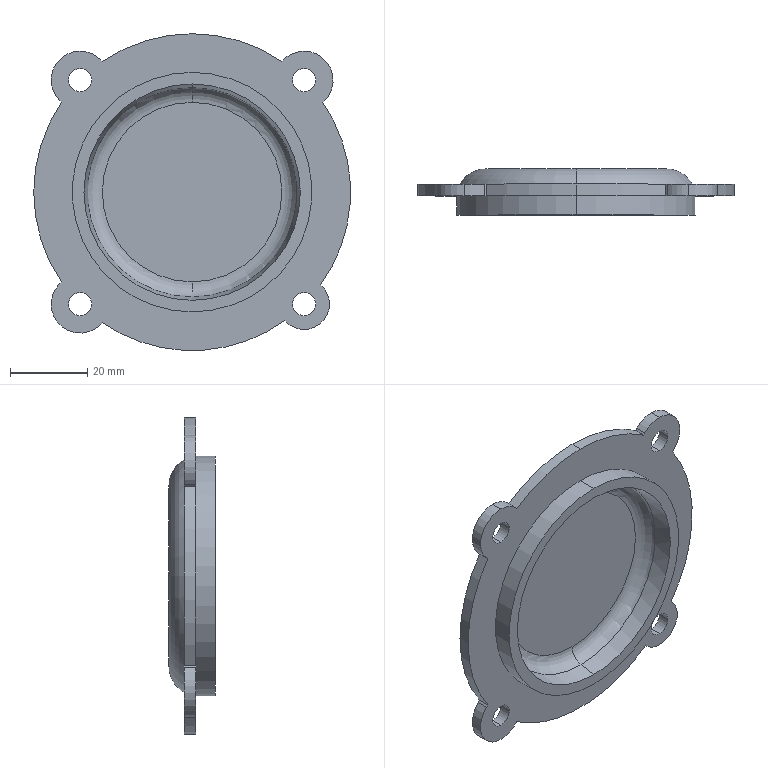Part | SolidWorks | features ICE 2, Revolution 1 | 1 solid | 40 faces | box 82 x 12 x 82 mm | volume 23262 mm3 | cylinder 21 | plane 13 | torus 4 | cone 2 | commonest cylinder face diameters 6 x8 15 x5 82 x5 62 x2 13.12 x1
STEP:
#1=CARTESIAN_POINT('',(-28.991,5.,25.991));
#2=VERTEX_POINT('',#1);
#3=CARTESIAN_POINT('',(-28.991,5.,31.991));
#4=VERTEX_POINT('',#3);
#5=CARTESIAN_POINT('',(-28.991,5.,28.991));
#6=DIRECTION('',(0.,1.,0.));
#7=DIRECTION('',(0.,0.,1.));
#8=AXIS2_PLACEMENT_3D('',#5,#6,#7);
#9=CIRCLE('',#8,3.);
#10=EDGE_CURVE('',#2,#4,#9,.T.);
#11=ORIENTED_EDGE('',*,*,#10,.F.);
#12=CARTESIAN_POINT('',(-28.991,8.,25.991));
#13=VERTEX_POINT('',#12);
#14=CARTESIAN_POINT('',(-28.991,0.,25.991));
#15=DIRECTION('',(0.,1.,0.));
#16=VECTOR('',#15,1000.);
#17=LINE('',#14,#16);
#18=EDGE_CURVE('',#2,#13,#17,.T.);
#19=ORIENTED_EDGE('',*,*,#18,.T.);
#20=CARTESIAN_POINT('',(-28.991,8.,31.991));
#21=VERTEX_POINT('',#20);
#22=CARTESIAN_POINT('',(-28.991,8.,28.991));
#23=DIRECTION('',(0.,1.,0.));
#24=DIRECTION('',(0.,0.,1.));
#25=AXIS2_PLACEMENT_3D('',#22,#23,#24);
#26=CIRCLE('',#25,3.);
#27=EDGE_CURVE('',#13,#21,#26,.T.);
#28=ORIENTED_EDGE('',*,*,#27,.T.);
#29=CARTESIAN_POINT('',(-28.991,0.,31.991));
#30=DIRECTION('',(0.,1.,0.));
#31=VECTOR('',#30,1000.);
#32=LINE('',#29,#31);
#33=EDGE_CURVE('',#4,#21,#32,.T.);
#34=ORIENTED_EDGE('',*,*,#33,.F.);
#35=EDGE_LOOP('',(#11,#19,#28,#34));
#36=FACE_OUTER_BOUND('',#35,.T.);
#37=CARTESIAN_POINT('',(-28.991,0.,28.991));
#38=DIRECTION('',(0.,1.,0.));
#39=DIRECTION('',(0.,0.,1.));
#40=AXIS2_PLACEMENT_3D('',#37,#38,#39);
#41=CYLINDRICAL_SURFACE('',#40,3.);
#42=ADVANCED_FACE('',(#36),#41,.F.);
#43=CARTESIAN_POINT('',(28.991,5.,25.991));
#44=VERTEX_POINT('',#43);
#45=CARTESIAN_POINT('',(28.991,5.,31.991));
#46=VERTEX_POINT('',#45);
#47=CARTESIAN_POINT('',(28.991,5.,28.991));
#48=DIRECTION('',(0.,1.,0.));
#49=DIRECTION('',(0.,0.,1.));
#50=AXIS2_PLACEMENT_3D('',#47,#48,#49);
#51=CIRCLE('',#50,3.);
#52=EDGE_CURVE('',#44,#46,#51,.T.);
#53=ORIENTED_EDGE('',*,*,#52,.F.);
#54=CARTESIAN_POINT('',(28.991,8.,25.991));
#55=VERTEX_POINT('',#54);
#56=CARTESIAN_POINT('',(28.991,0.,25.991));
#57=DIRECTION('',(0.,1.,0.));
#58=VECTOR('',#57,1000.);
#59=LINE('',#56,#58);
#60=EDGE_CURVE('',#44,#55,#59,.T.);
#61=ORIENTED_EDGE('',*,*,#60,.T.);
#62=CARTESIAN_POINT('',(28.991,8.,31.991));
#63=VERTEX_POINT('',#62);
#64=CARTESIAN_POINT('',(28.991,8.,28.991));
#65=DIRECTION('',(0.,1.,0.));
#66=DIRECTION('',(0.,0.,1.));
#67=AXIS2_PLACEMENT_3D('',#64,#65,#66);
#68=CIRCLE('',#67,3.);
#69=EDGE_CURVE('',#55,#63,#68,.T.);
#70=ORIENTED_EDGE('',*,*,#69,.T.);
#71=CARTESIAN_POINT('',(28.991,0.,31.991));
#72=DIRECTION('',(0.,1.,0.));
#73=VECTOR('',#72,1000.);
#74=LINE('',#71,#73);
#75=EDGE_CURVE('',#46,#63,#74,.T.);
#76=ORIENTED_EDGE('',*,*,#75,.F.);
#77=EDGE_LOOP('',(#53,#61,#70,#76));
#78=FACE_OUTER_BOUND('',#77,.T.);
#79=CARTESIAN_POINT('',(28.991,0.,28.991));
#80=DIRECTION('',(0.,1.,0.));
#81=DIRECTION('',(0.,0.,1.));
#82=AXIS2_PLACEMENT_3D('',#79,#80,#81);
#83=CYLINDRICAL_SURFACE('',#82,3.);
#84=ADVANCED_FACE('',(#78),#83,.F.);
#85=CARTESIAN_POINT('',(28.991,5.,-31.991));
#86=VERTEX_POINT('',#85);
#87=CARTESIAN_POINT('',(28.991,5.,-25.991));
#88=VERTEX_POINT('',#87);
#89=CARTESIAN_POINT('',(28.991,5.,-28.991));
#90=DIRECTION('',(0.,1.,0.));
#91=DIRECTION('',(0.,0.,1.));
#92=AXIS2_PLACEMENT_3D('',#89,#90,#91);
#93=CIRCLE('',#92,3.);
#94=EDGE_CURVE('',#86,#88,#93,.T.);
#95=ORIENTED_EDGE('',*,*,#94,.F.);
#96=CARTESIAN_POINT('',(28.991,8.,-31.991));
#97=VERTEX_POINT('',#96);
#98=CARTESIAN_POINT('',(28.991,0.,-31.991));
#99=DIRECTION('',(0.,1.,0.));
#100=VECTOR('',#99,1000.);
#101=LINE('',#98,#100);
#102=EDGE_CURVE('',#86,#97,#101,.T.);
#103=ORIENTED_EDGE('',*,*,#102,.T.);
#104=CARTESIAN_POINT('',(28.991,8.,-25.991));
#105=VERTEX_POINT('',#104);
#106=CARTESIAN_POINT('',(28.991,8.,-28.991));
#107=DIRECTION('',(0.,1.,0.));
#108=DIRECTION('',(0.,0.,1.));
#109=AXIS2_PLACEMENT_3D('',#106,#107,#108);
#110=CIRCLE('',#109,3.);
#111=EDGE_CURVE('',#97,#105,#110,.T.);
#112=ORIENTED_EDGE('',*,*,#111,.T.);
#113=CARTESIAN_POINT('',(28.991,0.,-25.991));
#114=DIRECTION('',(0.,1.,0.));
#115=VECTOR('',#114,1000.);
#116=LINE('',#113,#115);
#117=EDGE_CURVE('',#88,#105,#116,.T.);
#118=ORIENTED_EDGE('',*,*,#117,.F.);
#119=EDGE_LOOP('',(#95,#103,#112,#118));
#120=FACE_OUTER_BOUND('',#119,.T.);
#121=CARTESIAN_POINT('',(28.991,0.,-28.991));
#122=DIRECTION('',(0.,1.,0.));
#123=DIRECTION('',(0.,0.,1.));
#124=AXIS2_PLACEMENT_3D('',#121,#122,#123);
#125=CYLINDRICAL_SURFACE('',#124,3.);
#126=ADVANCED_FACE('',(#120),#125,.F.);
#127=CARTESIAN_POINT('',(-28.991,5.,-31.991));
#128=VERTEX_POINT('',#127);
#129=CARTESIAN_POINT('',(-28.991,5.,-25.991));
#130=VERTEX_POINT('',#129);
#131=CARTESIAN_POINT('',(-28.991,5.,-28.991));
#132=DIRECTION('',(0.,1.,0.));
#133=DIRECTION('',(0.,0.,1.));
#134=AXIS2_PLACEMENT_3D('',#131,#132,#133);
#135=CIRCLE('',#134,3.);
#136=EDGE_CURVE('',#128,#130,#135,.T.);
#137=ORIENTED_EDGE('',*,*,#136,.F.);
#138=CARTESIAN_POINT('',(-28.991,8.,-31.991));
#139=VERTEX_POINT('',#138);
#140=CARTESIAN_POINT('',(-28.991,0.,-31.991));
#141=DIRECTION('',(0.,1.,0.));
#142=VECTOR('',#141,1000.);
#143=LINE('',#140,#142);
#144=EDGE_CURVE('',#128,#139,#143,.T.);
#145=ORIENTED_EDGE('',*,*,#144,.T.);
#146=CARTESIAN_POINT('',(-28.991,8.,-25.991));
#147=VERTEX_POINT('',#146);
#148=CARTESIAN_POINT('',(-28.991,8.,-28.991));
#149=DIRECTION('',(0.,1.,0.));
#150=DIRECTION('',(0.,0.,1.));
#151=AXIS2_PLACEMENT_3D('',#148,#149,#150);
#152=CIRCLE('',#151,3.);
#153=EDGE_CURVE('',#139,#147,#152,.T.);
#154=ORIENTED_EDGE('',*,*,#153,.T.);
#155=CARTESIAN_POINT('',(-28.991,0.,-25.991));
#156=DIRECTION('',(0.,1.,0.));
#157=VECTOR('',#156,1000.);
#158=LINE('',#155,#157);
#159=EDGE_CURVE('',#130,#147,#158,.T.);
#160=ORIENTED_EDGE('',*,*,#159,.F.);
#161=EDGE_LOOP('',(#137,#145,#154,#160));
#162=FACE_OUTER_BOUND('',#161,.T.);
#163=CARTESIAN_POINT('',(-28.991,0.,-28.991));
#164=DIRECTION('',(0.,1.,0.));
#165=DIRECTION('',(0.,0.,1.));
#166=AXIS2_PLACEMENT_3D('',#163,#164,#165);
#167=CYLINDRICAL_SURFACE('',#166,3.);
#168=ADVANCED_FACE('',(#162),#167,.F.);
#169=CARTESIAN_POINT('',(23.681,5.,34.287));
#170=VERTEX_POINT('',#169);
#171=CARTESIAN_POINT('',(28.991,5.,36.491));
#172=VERTEX_POINT('',#171);
#173=CARTESIAN_POINT('',(28.991,5.,28.991));
#174=DIRECTION('',(0.,1.,0.));
#175=DIRECTION('',(0.,0.,1.));
#176=AXIS2_PLACEMENT_3D('',#173,#174,#175);
#177=CIRCLE('',#176,7.5);
#178=EDGE_CURVE('',#170,#172,#177,.T.);
#179=ORIENTED_EDGE('',*,*,#178,.T.);
#180=CARTESIAN_POINT('',(28.991,8.,36.491));
#181=VERTEX_POINT('',#180);
#182=CARTESIAN_POINT('',(28.991,5.,36.491));
#183=DIRECTION('',(0.,1.,0.));
#184=VECTOR('',#183,1000.);
#185=LINE('',#182,#184);
#186=EDGE_CURVE('',#172,#181,#185,.T.);
#187=ORIENTED_EDGE('',*,*,#186,.T.);
#188=CARTESIAN_POINT('',(23.681,8.,34.287));
#189=VERTEX_POINT('',#188);
#190=CARTESIAN_POINT('',(28.991,8.,28.991));
#191=DIRECTION('',(0.,1.,0.));
#192=DIRECTION('',(0.,0.,1.));
#193=AXIS2_PLACEMENT_3D('',#190,#191,#192);
#194=CIRCLE('',#193,7.5);
#195=EDGE_CURVE('',#189,#181,#194,.T.);
#196=ORIENTED_EDGE('',*,*,#195,.F.);
#197=CARTESIAN_POINT('',(23.681,5.,34.287));
#198=DIRECTION('',(0.,1.,0.));
#199=VECTOR('',#198,1000.);
#200=LINE('',#197,#199);
#201=EDGE_CURVE('',#170,#189,#200,.T.);
#202=ORIENTED_EDGE('',*,*,#201,.F.);
#203=EDGE_LOOP('',(#179,#187,#196,#202));
#204=FACE_OUTER_BOUND('',#203,.T.);
#205=CARTESIAN_POINT('',(28.991,5.,28.991));
#206=DIRECTION('',(0.,1.,0.));
#207=DIRECTION('',(0.,0.,1.));
#208=AXIS2_PLACEMENT_3D('',#205,#206,#207);
#209=CYLINDRICAL_SURFACE('',#208,7.5);
#210=ADVANCED_FACE('',(#204),#209,.T.);
#211=CARTESIAN_POINT('',(-34.234,5.,23.628));
#212=VERTEX_POINT('',#211);
#213=CARTESIAN_POINT('',(-28.991,5.,36.491));
#214=VERTEX_POINT('',#213);
#215=CARTESIAN_POINT('',(-28.991,5.,28.991));
#216=DIRECTION('',(0.,1.,0.));
#217=DIRECTION('',(0.,0.,1.));
#218=AXIS2_PLACEMENT_3D('',#215,#216,#217);
#219=CIRCLE('',#218,7.5);
#220=EDGE_CURVE('',#212,#214,#219,.T.);
#221=ORIENTED_EDGE('',*,*,#220,.T.);
#222=CARTESIAN_POINT('',(-28.991,8.,36.491));
#223=VERTEX_POINT('',#222);
#224=CARTESIAN_POINT('',(-28.991,5.,36.491));
#225=DIRECTION('',(0.,1.,0.));
#226=VECTOR('',#225,1000.);
#227=LINE('',#224,#226);
#228=EDGE_CURVE('',#214,#223,#227,.T.);
#229=ORIENTED_EDGE('',*,*,#228,.T.);
#230=CARTESIAN_POINT('',(-34.234,8.,23.628));
#231=VERTEX_POINT('',#230);
#232=CARTESIAN_POINT('',(-28.991,8.,28.991));
#233=DIRECTION('',(0.,1.,0.));
#234=DIRECTION('',(0.,0.,1.));
#235=AXIS2_PLACEMENT_3D('',#232,#233,#234);
#236=CIRCLE('',#235,7.5);
#237=EDGE_CURVE('',#231,#223,#236,.T.);
#238=ORIENTED_EDGE('',*,*,#237,.F.);
#239=CARTESIAN_POINT('',(-34.234,5.,23.628));
#240=DIRECTION('',(0.,1.,0.));
#241=VECTOR('',#240,1000.);
#242=LINE('',#239,#241);
#243=EDGE_CURVE('',#212,#231,#242,.T.);
#244=ORIENTED_EDGE('',*,*,#243,.F.);
#245=EDGE_LOOP('',(#221,#229,#238,#244));
#246=FACE_OUTER_BOUND('',#245,.T.);
#247=CARTESIAN_POINT('',(-28.991,5.,28.991));
#248=DIRECTION('',(0.,1.,0.));
#249=DIRECTION('',(0.,0.,1.));
#250=AXIS2_PLACEMENT_3D('',#247,#248,#249);
#251=CYLINDRICAL_SURFACE('',#250,7.5);
#252=ADVANCED_FACE('',(#246),#251,.T.);
#253=CARTESIAN_POINT('',(0.,4.695,-27.172));
#254=VERTEX_POINT('',#253);
#255=CARTESIAN_POINT('',(0.,4.695,27.172));
#256=VERTEX_POINT('',#255);
#257=CARTESIAN_POINT('',(0.,4.695,0.));
#258=DIRECTION('',(0.,1.,0.));
#259=DIRECTION('',(0.,0.,1.));
#260=AXIS2_PLACEMENT_3D('',#257,#258,#259);
#261=CIRCLE('',#260,27.172);
#262=EDGE_CURVE('',#254,#256,#261,.T.);
#263=ORIENTED_EDGE('',*,*,#262,.F.);
#264=CARTESIAN_POINT('',(0.,8.,-23.233));
#265=VERTEX_POINT('',#264);
#266=CARTESIAN_POINT('',(0.,4.,-23.233));
#267=DIRECTION('',(1.,0.,0.));
#268=DIRECTION('',(0.,0.,-1.));
#269=AXIS2_PLACEMENT_3D('',#266,#267,#268);
#270=CIRCLE('',#269,4.);
#271=EDGE_CURVE('',#254,#265,#270,.T.);
#272=ORIENTED_EDGE('',*,*,#271,.T.);
#273=CARTESIAN_POINT('',(0.,8.,23.233));
#274=VERTEX_POINT('',#273);
#275=CARTESIAN_POINT('',(0.,8.,0.));
#276=DIRECTION('',(0.,1.,0.));
#277=DIRECTION('',(0.,0.,1.));
#278=AXIS2_PLACEMENT_3D('',#275,#276,#277);
#279=CIRCLE('',#278,23.233);
#280=EDGE_CURVE('',#265,#274,#279,.T.);
#281=ORIENTED_EDGE('',*,*,#280,.T.);
#282=CARTESIAN_POINT('',(0.,4.,23.233));
#283=DIRECTION('',(-1.,0.,0.));
#284=DIRECTION('',(0.,0.,1.));
#285=AXIS2_PLACEMENT_3D('',#282,#283,#284);
#286=CIRCLE('',#285,4.);
#287=EDGE_CURVE('',#256,#274,#286,.T.);
#288=ORIENTED_EDGE('',*,*,#287,.F.);
#289=EDGE_LOOP('',(#263,#272,#281,#288));
#290=FACE_OUTER_BOUND('',#289,.T.);
#291=CARTESIAN_POINT('',(0.,4.,0.));
#292=DIRECTION('',(0.,1.,0.));
#293=DIRECTION('',(0.,0.,1.));
#294=AXIS2_PLACEMENT_3D('',#291,#292,#293);
#295=TOROIDAL_SURFACE('',#294,23.233,4.);
#296=ADVANCED_FACE('',(#290),#295,.F.);
#297=CARTESIAN_POINT('',(0.,8.,30.161));
#298=VERTEX_POINT('',#297);
#299=CARTESIAN_POINT('',(0.,8.,-30.161));
#300=VERTEX_POINT('',#299);
#301=CARTESIAN_POINT('',(0.,8.,0.));
#302=DIRECTION('',(0.,1.,0.));
#303=DIRECTION('',(0.,0.,1.));
#304=AXIS2_PLACEMENT_3D('',#301,#302,#303);
#305=CIRCLE('',#304,30.161);
#306=EDGE_CURVE('',#298,#300,#305,.T.);
#307=ORIENTED_EDGE('',*,*,#306,.T.);
#308=CARTESIAN_POINT('',(0.,12.,-23.233));
#309=VERTEX_POINT('',#308);
#310=CARTESIAN_POINT('',(0.,4.,-23.233));
#311=DIRECTION('',(1.,0.,0.));
#312=DIRECTION('',(0.,0.,-1.));
#313=AXIS2_PLACEMENT_3D('',#310,#311,#312);
#314=CIRCLE('',#313,8.);
#315=EDGE_CURVE('',#300,#309,#314,.T.);
#316=ORIENTED_EDGE('',*,*,#315,.T.);
#317=CARTESIAN_POINT('',(0.,12.,23.233));
#318=VERTEX_POINT('',#317);
#319=CARTESIAN_POINT('',(0.,12.,0.));
#320=DIRECTION('',(0.,1.,0.));
#321=DIRECTION('',(0.,0.,1.));
#322=AXIS2_PLACEMENT_3D('',#319,#320,#321);
#323=CIRCLE('',#322,23.233);
#324=EDGE_CURVE('',#318,#309,#323,.T.);
#325=ORIENTED_EDGE('',*,*,#324,.F.);
#326=CARTESIAN_POINT('',(0.,4.,23.233));
#327=DIRECTION('',(-1.,0.,0.));
#328=DIRECTION('',(0.,0.,1.));
#329=AXIS2_PLACEMENT_3D('',#326,#327,#328);
#330=CIRCLE('',#329,8.);
#331=EDGE_CURVE('',#298,#318,#330,.T.);
#332=ORIENTED_EDGE('',*,*,#331,.F.);
#333=EDGE_LOOP('',(#307,#316,#325,#332));
#334=FACE_OUTER_BOUND('',#333,.T.);
#335=CARTESIAN_POINT('',(0.,4.,0.));
#336=DIRECTION('',(0.,1.,0.));
#337=DIRECTION('',(0.,0.,1.));
#338=AXIS2_PLACEMENT_3D('',#335,#336,#337);
#339=TOROIDAL_SURFACE('',#338,23.233,8.);
#340=ADVANCED_FACE('',(#334),#339,.T.);
#341=CARTESIAN_POINT('',(0.,0.,31.));
#342=VERTEX_POINT('',#341);
#343=CARTESIAN_POINT('',(0.,0.,-31.));
#344=VERTEX_POINT('',#343);
#345=CARTESIAN_POINT('',(0.,0.,0.));
#346=DIRECTION('',(0.,1.,0.));
#347=DIRECTION('',(0.,0.,1.));
#348=AXIS2_PLACEMENT_3D('',#345,#346,#347);
#349=CIRCLE('',#348,31.);
#350=EDGE_CURVE('',#342,#344,#349,.T.);
#351=ORIENTED_EDGE('',*,*,#350,.T.);
#352=CARTESIAN_POINT('',(0.,5.,-31.));
#353=VERTEX_POINT('',#352);
#354=CARTESIAN_POINT('',(0.,53.941,-31.));
#355=DIRECTION('',(0.,1.,0.));
#356=VECTOR('',#355,1000.);
#357=LINE('',#354,#356);
#358=EDGE_CURVE('',#344,#353,#357,.T.);
#359=ORIENTED_EDGE('',*,*,#358,.T.);
#360=CARTESIAN_POINT('',(0.,5.,31.));
#361=VERTEX_POINT('',#360);
#362=CARTESIAN_POINT('',(0.,5.,0.));
#363=DIRECTION('',(0.,1.,0.));
#364=DIRECTION('',(0.,0.,1.));
#365=AXIS2_PLACEMENT_3D('',#362,#363,#364);
#366=CIRCLE('',#365,31.);
#367=EDGE_CURVE('',#361,#353,#366,.T.);
#368=ORIENTED_EDGE('',*,*,#367,.F.);
#369=CARTESIAN_POINT('',(0.,53.941,31.));
#370=DIRECTION('',(0.,1.,0.));
#371=VECTOR('',#370,1000.);
#372=LINE('',#369,#371);
#373=EDGE_CURVE('',#342,#361,#372,.T.);
#374=ORIENTED_EDGE('',*,*,#373,.F.);
#375=EDGE_LOOP('',(#351,#359,#368,#374));
#376=FACE_OUTER_BOUND('',#375,.T.);
#377=CARTESIAN_POINT('',(0.,53.941,0.));
#378=DIRECTION('',(0.,1.,0.));
#379=DIRECTION('',(0.,0.,1.));
#380=AXIS2_PLACEMENT_3D('',#377,#378,#379);
#381=CYLINDRICAL_SURFACE('',#380,31.);
#382=ADVANCED_FACE('',(#376),#381,.T.);
#383=ORIENTED_EDGE('',*,*,#262,.T.);
#384=CARTESIAN_POINT('',(0.,0.,28.));
#385=VERTEX_POINT('',#384);
#386=CARTESIAN_POINT('',(0.,4.695,27.172));
#387=DIRECTION('',(0.,-0.9848,0.1736));
#388=VECTOR('',#387,1000.);
#389=LINE('',#386,#388);
#390=EDGE_CURVE('',#256,#385,#389,.T.);
#391=ORIENTED_EDGE('',*,*,#390,.T.);
#392=CARTESIAN_POINT('',(0.,0.,-28.));
#393=VERTEX_POINT('',#392);
#394=CARTESIAN_POINT('',(0.,0.,0.));
#395=DIRECTION('',(0.,1.,0.));
#396=DIRECTION('',(0.,0.,1.));
#397=AXIS2_PLACEMENT_3D('',#394,#395,#396);
#398=CIRCLE('',#397,28.);
#399=EDGE_CURVE('',#393,#385,#398,.T.);
#400=ORIENTED_EDGE('',*,*,#399,.F.);
#401=CARTESIAN_POINT('',(0.,4.695,-27.172));
#402=DIRECTION('',(0.,-0.9848,-0.1736));
#403=VECTOR('',#402,1000.);
#404=LINE('',#401,#403);
#405=EDGE_CURVE('',#254,#393,#404,.T.);
#406=ORIENTED_EDGE('',*,*,#405,.F.);
#407=EDGE_LOOP('',(#383,#391,#400,#406));
#408=FACE_OUTER_BOUND('',#407,.T.);
#409=CARTESIAN_POINT('',(0.,4.695,0.));
#410=DIRECTION('',(0.,-1.,0.));
#411=DIRECTION('',(0.,0.,-1.));
#412=AXIS2_PLACEMENT_3D('',#409,#410,#411);
#413=CONICAL_SURFACE('',#412,27.172,0.1745);
#414=ADVANCED_FACE('',(#408),#413,.F.);
#415=CARTESIAN_POINT('',(-23.205,5.,33.801));
#416=VERTEX_POINT('',#415);
#417=CARTESIAN_POINT('',(0.,5.,41.));
#418=VERTEX_POINT('',#417);
#419=CARTESIAN_POINT('',(0.,5.,0.));
#420=DIRECTION('',(0.,1.,0.));
#421=DIRECTION('',(0.,0.,1.));
#422=AXIS2_PLACEMENT_3D('',#419,#420,#421);
#423=CIRCLE('',#422,41.);
#424=EDGE_CURVE('',#416,#418,#423,.T.);
#425=ORIENTED_EDGE('',*,*,#424,.T.);
#426=CARTESIAN_POINT('',(0.,8.,41.));
#427=VERTEX_POINT('',#426);
#428=CARTESIAN_POINT('',(0.,53.941,41.));
#429=DIRECTION('',(0.,1.,0.));
#430=VECTOR('',#429,1000.);
#431=LINE('',#428,#430);
#432=EDGE_CURVE('',#418,#427,#431,.T.);
#433=ORIENTED_EDGE('',*,*,#432,.T.);
#434=CARTESIAN_POINT('',(-23.205,8.,33.801));
#435=VERTEX_POINT('',#434);
#436=CARTESIAN_POINT('',(0.,8.,0.));
#437=DIRECTION('',(0.,1.,0.));
#438=DIRECTION('',(0.,0.,1.));
#439=AXIS2_PLACEMENT_3D('',#436,#437,#438);
#440=CIRCLE('',#439,41.);
#441=EDGE_CURVE('',#435,#427,#440,.T.);
#442=ORIENTED_EDGE('',*,*,#441,.F.);
#443=CARTESIAN_POINT('',(-23.205,5.,33.801));
#444=DIRECTION('',(0.,1.,0.));
#445=VECTOR('',#444,1000.);
#446=LINE('',#443,#445);
#447=EDGE_CURVE('',#416,#435,#446,.T.);
#448=ORIENTED_EDGE('',*,*,#447,.F.);
#449=EDGE_LOOP('',(#425,#433,#442,#448));
#450=FACE_OUTER_BOUND('',#449,.T.);
#451=CARTESIAN_POINT('',(0.,53.941,0.));
#452=DIRECTION('',(0.,1.,0.));
#453=DIRECTION('',(0.,0.,1.));
#454=AXIS2_PLACEMENT_3D('',#451,#452,#453);
#455=CYLINDRICAL_SURFACE('',#454,41.);
#456=ADVANCED_FACE('',(#450),#455,.T.);
#457=ORIENTED_EDGE('',*,*,#432,.F.);
#458=CARTESIAN_POINT('',(23.199,5.,33.805));
#459=VERTEX_POINT('',#458);
#460=CARTESIAN_POINT('',(0.,5.,0.));
#461=DIRECTION('',(0.,1.,0.));
#462=DIRECTION('',(0.,0.,1.));
#463=AXIS2_PLACEMENT_3D('',#460,#461,#462);
#464=CIRCLE('',#463,41.);
#465=EDGE_CURVE('',#418,#459,#464,.T.);
#466=ORIENTED_EDGE('',*,*,#465,.T.);
#467=CARTESIAN_POINT('',(23.199,8.,33.805));
#468=VERTEX_POINT('',#467);
#469=CARTESIAN_POINT('',(23.199,5.,33.805));
#470=DIRECTION('',(0.,1.,0.));
#471=VECTOR('',#470,1000.);
#472=LINE('',#469,#471);
#473=EDGE_CURVE('',#459,#468,#472,.T.);
#474=ORIENTED_EDGE('',*,*,#473,.T.);
#475=CARTESIAN_POINT('',(0.,8.,0.));
#476=DIRECTION('',(0.,1.,0.));
#477=DIRECTION('',(0.,0.,1.));
#478=AXIS2_PLACEMENT_3D('',#475,#476,#477);
#479=CIRCLE('',#478,41.);
#480=EDGE_CURVE('',#427,#468,#479,.T.);
#481=ORIENTED_EDGE('',*,*,#480,.F.);
#482=EDGE_LOOP('',(#457,#466,#474,#481));
#483=FACE_OUTER_BOUND('',#482,.T.);
#484=CARTESIAN_POINT('',(0.,53.941,0.));
#485=DIRECTION('',(0.,1.,0.));
#486=DIRECTION('',(0.,0.,1.));
#487=AXIS2_PLACEMENT_3D('',#484,#485,#486);
#488=CYLINDRICAL_SURFACE('',#487,41.);
#489=ADVANCED_FACE('',(#483),#488,.T.);
#490=CARTESIAN_POINT('',(-33.805,5.,-23.199));
#491=VERTEX_POINT('',#490);
#492=CARTESIAN_POINT('',(-33.801,5.,23.205));
#493=VERTEX_POINT('',#492);
#494=CARTESIAN_POINT('',(0.,5.,0.));
#495=DIRECTION('',(0.,1.,0.));
#496=DIRECTION('',(0.,0.,1.));
#497=AXIS2_PLACEMENT_3D('',#494,#495,#496);
#498=CIRCLE('',#497,41.);
#499=EDGE_CURVE('',#491,#493,#498,.T.);
#500=ORIENTED_EDGE('',*,*,#499,.T.);
#501=CARTESIAN_POINT('',(-33.801,8.,23.205));
#502=VERTEX_POINT('',#501);
#503=CARTESIAN_POINT('',(-33.801,5.,23.205));
#504=DIRECTION('',(0.,1.,0.));
#505=VECTOR('',#504,1000.);
#506=LINE('',#503,#505);
#507=EDGE_CURVE('',#493,#502,#506,.T.);
#508=ORIENTED_EDGE('',*,*,#507,.T.);
#509=CARTESIAN_POINT('',(-33.805,8.,-23.199));
#510=VERTEX_POINT('',#509);
#511=CARTESIAN_POINT('',(0.,8.,0.));
#512=DIRECTION('',(0.,1.,0.));
#513=DIRECTION('',(0.,0.,1.));
#514=AXIS2_PLACEMENT_3D('',#511,#512,#513);
#515=CIRCLE('',#514,41.);
#516=EDGE_CURVE('',#510,#502,#515,.T.);
#517=ORIENTED_EDGE('',*,*,#516,.F.);
#518=CARTESIAN_POINT('',(-33.805,5.,-23.199));
#519=DIRECTION('',(0.,1.,0.));
#520=VECTOR('',#519,1000.);
#521=LINE('',#518,#520);
#522=EDGE_CURVE('',#491,#510,#521,.T.);
#523=ORIENTED_EDGE('',*,*,#522,.F.);
#524=EDGE_LOOP('',(#500,#508,#517,#523));
#525=FACE_OUTER_BOUND('',#524,.T.);
#526=CARTESIAN_POINT('',(0.,53.941,0.));
#527=DIRECTION('',(0.,1.,0.));
#528=DIRECTION('',(0.,0.,1.));
#529=AXIS2_PLACEMENT_3D('',#526,#527,#528);
#530=CYLINDRICAL_SURFACE('',#529,41.);
#531=ADVANCED_FACE('',(#525),#530,.T.);
#532=CARTESIAN_POINT('',(23.974,5.,-33.26));
#533=VERTEX_POINT('',#532);
#534=CARTESIAN_POINT('',(-23.204,5.,-33.802));
#535=VERTEX_POINT('',#534);
#536=CARTESIAN_POINT('',(0.,5.,0.));
#537=DIRECTION('',(0.,1.,0.));
#538=DIRECTION('',(0.,0.,1.));
#539=AXIS2_PLACEMENT_3D('',#536,#537,#538);
#540=CIRCLE('',#539,41.);
#541=EDGE_CURVE('',#533,#535,#540,.T.);
#542=ORIENTED_EDGE('',*,*,#541,.T.);
#543=CARTESIAN_POINT('',(-23.204,8.,-33.802));
#544=VERTEX_POINT('',#543);
#545=CARTESIAN_POINT('',(-23.204,5.,-33.802));
#546=DIRECTION('',(0.,1.,0.));
#547=VECTOR('',#546,1000.);
#548=LINE('',#545,#547);
#549=EDGE_CURVE('',#535,#544,#548,.T.);
#550=ORIENTED_EDGE('',*,*,#549,.T.);
#551=CARTESIAN_POINT('',(23.974,8.,-33.26));
#552=VERTEX_POINT('',#551);
#553=CARTESIAN_POINT('',(0.,8.,0.));
#554=DIRECTION('',(0.,1.,0.));
#555=DIRECTION('',(0.,0.,1.));
#556=AXIS2_PLACEMENT_3D('',#553,#554,#555);
#557=CIRCLE('',#556,41.);
#558=EDGE_CURVE('',#552,#544,#557,.T.);
#559=ORIENTED_EDGE('',*,*,#558,.F.);
#560=CARTESIAN_POINT('',(23.974,5.,-33.26));
#561=DIRECTION('',(0.,1.,0.));
#562=VECTOR('',#561,1000.);
#563=LINE('',#560,#562);
#564=EDGE_CURVE('',#533,#552,#563,.T.);
#565=ORIENTED_EDGE('',*,*,#564,.F.);
#566=EDGE_LOOP('',(#542,#550,#559,#565));
#567=FACE_OUTER_BOUND('',#566,.T.);
#568=CARTESIAN_POINT('',(0.,53.941,0.));
#569=DIRECTION('',(0.,1.,0.));
#570=DIRECTION('',(0.,0.,1.));
#571=AXIS2_PLACEMENT_3D('',#568,#569,#570);
#572=CYLINDRICAL_SURFACE('',#571,41.);
#573=ADVANCED_FACE('',(#567),#572,.T.);
#574=ORIENTED_EDGE('',*,*,#390,.F.);
#575=CARTESIAN_POINT('',(0.,4.695,0.));
#576=DIRECTION('',(0.,1.,0.));
#577=DIRECTION('',(0.,0.,1.));
#578=AXIS2_PLACEMENT_3D('',#575,#576,#577);
#579=CIRCLE('',#578,27.172);
#580=EDGE_CURVE('',#256,#254,#579,.T.);
#581=ORIENTED_EDGE('',*,*,#580,.T.);
#582=ORIENTED_EDGE('',*,*,#405,.T.);
#583=CARTESIAN_POINT('',(0.,0.,0.));
#584=DIRECTION('',(0.,1.,0.));
#585=DIRECTION('',(0.,0.,1.));
#586=AXIS2_PLACEMENT_3D('',#583,#584,#585);
#587=CIRCLE('',#586,28.);
#588=EDGE_CURVE('',#385,#393,#587,.T.);
#589=ORIENTED_EDGE('',*,*,#588,.F.);
#590=EDGE_LOOP('',(#574,#581,#582,#589));
#591=FACE_OUTER_BOUND('',#590,.T.);
#592=CARTESIAN_POINT('',(0.,4.695,0.));
#593=DIRECTION('',(0.,-1.,0.));
#594=DIRECTION('',(0.,0.,-1.));
#595=AXIS2_PLACEMENT_3D('',#592,#593,#594);
#596=CONICAL_SURFACE('',#595,27.172,0.1745);
#597=ADVANCED_FACE('',(#591),#596,.F.);
#598=ORIENTED_EDGE('',*,*,#350,.F.);
#599=CARTESIAN_POINT('',(0.,0.,0.));
#600=DIRECTION('',(0.,1.,0.));
#601=DIRECTION('',(0.,0.,1.));
#602=AXIS2_PLACEMENT_3D('',#599,#600,#601);
#603=CIRCLE('',#602,31.);
#604=EDGE_CURVE('',#344,#342,#603,.T.);
#605=ORIENTED_EDGE('',*,*,#604,.F.);
#606=EDGE_LOOP('',(#598,#605));
#607=FACE_OUTER_BOUND('',#606,.T.);
#608=ORIENTED_EDGE('',*,*,#399,.T.);
#609=ORIENTED_EDGE('',*,*,#588,.T.);
#610=EDGE_LOOP('',(#608,#609));
#611=FACE_BOUND('',#610,.T.);
#612=CARTESIAN_POINT('',(0.,0.,-28.));
#613=DIRECTION('',(0.,1.,0.));
#614=DIRECTION('',(0.,0.,1.));
#615=AXIS2_PLACEMENT_3D('',#612,#613,#614);
#616=PLANE('',#615);
#617=ADVANCED_FACE('',(#607,#611),#616,.F.);
#618=ORIENTED_EDGE('',*,*,#358,.F.);
#619=ORIENTED_EDGE('',*,*,#604,.T.);
#620=ORIENTED_EDGE('',*,*,#373,.T.);
#621=CARTESIAN_POINT('',(0.,5.,0.));
#622=DIRECTION('',(0.,1.,0.));
#623=DIRECTION('',(0.,0.,1.));
#624=AXIS2_PLACEMENT_3D('',#621,#622,#623);
#625=CIRCLE('',#624,31.);
#626=EDGE_CURVE('',#353,#361,#625,.T.);
#627=ORIENTED_EDGE('',*,*,#626,.F.);
#628=EDGE_LOOP('',(#618,#619,#620,#627));
#629=FACE_OUTER_BOUND('',#628,.T.);
#630=CARTESIAN_POINT('',(0.,53.941,0.));
#631=DIRECTION('',(0.,1.,0.));
#632=DIRECTION('',(0.,0.,1.));
#633=AXIS2_PLACEMENT_3D('',#630,#631,#632);
#634=CYLINDRICAL_SURFACE('',#633,31.);
#635=ADVANCED_FACE('',(#629),#634,.T.);
#636=CARTESIAN_POINT('',(-28.991,5.,28.991));
#637=DIRECTION('',(0.,1.,0.));
#638=DIRECTION('',(0.,0.,1.));
#639=AXIS2_PLACEMENT_3D('',#636,#637,#638);
#640=CIRCLE('',#639,3.);
#641=EDGE_CURVE('',#4,#2,#640,.T.);
#642=ORIENTED_EDGE('',*,*,#641,.T.);
#643=ORIENTED_EDGE('',*,*,#10,.T.);
#644=EDGE_LOOP('',(#642,#643));
#645=FACE_BOUND('',#644,.T.);
#646=CARTESIAN_POINT('',(28.991,5.,28.991));
#647=DIRECTION('',(0.,1.,0.));
#648=DIRECTION('',(0.,0.,1.));
#649=AXIS2_PLACEMENT_3D('',#646,#647,#648);
#650=CIRCLE('',#649,3.);
#651=EDGE_CURVE('',#46,#44,#650,.T.);
#652=ORIENTED_EDGE('',*,*,#651,.T.);
#653=ORIENTED_EDGE('',*,*,#52,.T.);
#654=EDGE_LOOP('',(#652,#653));
#655=FACE_BOUND('',#654,.T.);
#656=CARTESIAN_POINT('',(28.991,5.,-28.991));
#657=DIRECTION('',(0.,1.,0.));
#658=DIRECTION('',(0.,0.,1.));
#659=AXIS2_PLACEMENT_3D('',#656,#657,#658);
#660=CIRCLE('',#659,3.);
#661=EDGE_CURVE('',#88,#86,#660,.T.);
#662=ORIENTED_EDGE('',*,*,#661,.T.);
#663=ORIENTED_EDGE('',*,*,#94,.T.);
#664=EDGE_LOOP('',(#662,#663));
#665=FACE_BOUND('',#664,.T.);
#666=CARTESIAN_POINT('',(-28.991,5.,-28.991));
#667=DIRECTION('',(0.,1.,0.));
#668=DIRECTION('',(0.,0.,1.));
#669=AXIS2_PLACEMENT_3D('',#666,#667,#668);
#670=CIRCLE('',#669,3.);
#671=EDGE_CURVE('',#130,#128,#670,.T.);
#672=ORIENTED_EDGE('',*,*,#671,.T.);
#673=ORIENTED_EDGE('',*,*,#136,.T.);
#674=EDGE_LOOP('',(#672,#673));
#675=FACE_BOUND('',#674,.T.);
#676=CARTESIAN_POINT('',(33.805,5.,23.199));
#677=VERTEX_POINT('',#676);
#678=CARTESIAN_POINT('',(33.26,5.,-23.974));
#679=VERTEX_POINT('',#678);
#680=CARTESIAN_POINT('',(0.,5.,0.));
#681=DIRECTION('',(0.,1.,0.));
#682=DIRECTION('',(0.,0.,1.));
#683=AXIS2_PLACEMENT_3D('',#680,#681,#682);
#684=CIRCLE('',#683,41.);
#685=EDGE_CURVE('',#677,#679,#684,.T.);
#686=ORIENTED_EDGE('',*,*,#685,.F.);
#687=CARTESIAN_POINT('',(34.294,5.,23.688));
#688=VERTEX_POINT('',#687);
#689=CARTESIAN_POINT('',(34.294,5.,23.688));
#690=DIRECTION('',(-0.7072,0.,-0.7071));
#691=VECTOR('',#690,1000.);
#692=LINE('',#689,#691);
#693=EDGE_CURVE('',#688,#677,#692,.T.);
#694=ORIENTED_EDGE('',*,*,#693,.F.);
#695=CARTESIAN_POINT('',(28.991,5.,28.991));
#696=DIRECTION('',(0.,1.,0.));
#697=DIRECTION('',(0.,0.,1.));
#698=AXIS2_PLACEMENT_3D('',#695,#696,#697);
#699=CIRCLE('',#698,7.5);
#700=EDGE_CURVE('',#172,#688,#699,.T.);
#701=ORIENTED_EDGE('',*,*,#700,.F.);
#702=ORIENTED_EDGE('',*,*,#178,.F.);
#703=CARTESIAN_POINT('',(23.199,5.,33.805));
#704=DIRECTION('',(0.7071,0.,0.7071));
#705=VECTOR('',#704,1000.);
#706=LINE('',#703,#705);
#707=EDGE_CURVE('',#459,#170,#706,.T.);
#708=ORIENTED_EDGE('',*,*,#707,.F.);
#709=ORIENTED_EDGE('',*,*,#465,.F.);
#710=ORIENTED_EDGE('',*,*,#424,.F.);
#711=CARTESIAN_POINT('',(-23.628,5.,34.234));
#712=VERTEX_POINT('',#711);
#713=CARTESIAN_POINT('',(-23.205,5.,33.801));
#714=DIRECTION('',(0.699,0.,-0.7152));
#715=VECTOR('',#714,1000.);
#716=LINE('',#713,#715);
#717=EDGE_CURVE('',#712,#416,#716,.T.);
#718=ORIENTED_EDGE('',*,*,#717,.F.);
#719=CARTESIAN_POINT('',(-28.991,5.,28.991));
#720=DIRECTION('',(0.,1.,0.));
#721=DIRECTION('',(0.,0.,1.));
#722=AXIS2_PLACEMENT_3D('',#719,#720,#721);
#723=CIRCLE('',#722,7.5);
#724=EDGE_CURVE('',#214,#712,#723,.T.);
#725=ORIENTED_EDGE('',*,*,#724,.F.);
#726=ORIENTED_EDGE('',*,*,#220,.F.);
#727=CARTESIAN_POINT('',(-34.234,5.,23.628));
#728=DIRECTION('',(-0.7152,0.,0.699));
#729=VECTOR('',#728,1000.);
#730=LINE('',#727,#729);
#731=EDGE_CURVE('',#493,#212,#730,.T.);
#732=ORIENTED_EDGE('',*,*,#731,.F.);
#733=ORIENTED_EDGE('',*,*,#499,.F.);
#734=CARTESIAN_POINT('',(-34.295,5.,-23.688));
#735=VERTEX_POINT('',#734);
#736=CARTESIAN_POINT('',(-34.295,5.,-23.688));
#737=DIRECTION('',(0.7071,0.,0.7071));
#738=VECTOR('',#737,1000.);
#739=LINE('',#736,#738);
#740=EDGE_CURVE('',#735,#491,#739,.T.);
#741=ORIENTED_EDGE('',*,*,#740,.F.);
#742=CARTESIAN_POINT('',(-23.643,5.,-34.249));
#743=VERTEX_POINT('',#742);
#744=CARTESIAN_POINT('',(-28.991,5.,-28.991));
#745=DIRECTION('',(0.,1.,0.));
#746=DIRECTION('',(0.,0.,1.));
#747=AXIS2_PLACEMENT_3D('',#744,#745,#746);
#748=CIRCLE('',#747,7.5);
#749=EDGE_CURVE('',#743,#735,#748,.T.);
#750=ORIENTED_EDGE('',*,*,#749,.F.);
#751=CARTESIAN_POINT('',(-23.204,5.,-33.802));
#752=DIRECTION('',(-0.701,0.,-0.7131));
#753=VECTOR('',#752,1000.);
#754=LINE('',#751,#753);
#755=EDGE_CURVE('',#535,#743,#754,.T.);
#756=ORIENTED_EDGE('',*,*,#755,.F.);
#757=ORIENTED_EDGE('',*,*,#541,.F.);
#758=CARTESIAN_POINT('',(24.406,5.,-33.683));
#759=VERTEX_POINT('',#758);
#760=CARTESIAN_POINT('',(23.974,5.,-33.26));
#761=DIRECTION('',(-0.7152,0.,0.699));
#762=VECTOR('',#761,1000.);
#763=LINE('',#760,#762);
#764=EDGE_CURVE('',#759,#533,#763,.T.);
#765=ORIENTED_EDGE('',*,*,#764,.F.);
#766=CARTESIAN_POINT('',(33.683,5.,-24.406));
#767=VERTEX_POINT('',#766);
#768=CARTESIAN_POINT('',(28.991,5.,-28.991));
#769=DIRECTION('',(0.,1.,0.));
#770=DIRECTION('',(0.,0.,1.));
#771=AXIS2_PLACEMENT_3D('',#768,#769,#770);
#772=CIRCLE('',#771,6.56);
#773=EDGE_CURVE('',#767,#759,#772,.T.);
#774=ORIENTED_EDGE('',*,*,#773,.F.);
#775=CARTESIAN_POINT('',(33.683,5.,-24.406));
#776=DIRECTION('',(0.699,0.,-0.7152));
#777=VECTOR('',#776,1000.);
#778=LINE('',#775,#777);
#779=EDGE_CURVE('',#679,#767,#778,.T.);
#780=ORIENTED_EDGE('',*,*,#779,.F.);
#781=EDGE_LOOP('',(#686,#694,#701,#702,#708,#709,#710,#718,#725,#726,#732,#733,#741,#750,#756,#757,#765,#774,#780));
#782=FACE_OUTER_BOUND('',#781,.T.);
#783=ORIENTED_EDGE('',*,*,#367,.T.);
#784=ORIENTED_EDGE('',*,*,#626,.T.);
#785=EDGE_LOOP('',(#783,#784));
#786=FACE_BOUND('',#785,.T.);
#787=CARTESIAN_POINT('',(0.,5.,-31.));
#788=DIRECTION('',(0.,1.,0.));
#789=DIRECTION('',(0.,0.,1.));
#790=AXIS2_PLACEMENT_3D('',#787,#788,#789);
#791=PLANE('',#790);
#792=ADVANCED_FACE('',(#645,#655,#665,#675,#782,#786),#791,.F.);
#793=ORIENTED_EDGE('',*,*,#685,.T.);
#794=CARTESIAN_POINT('',(33.26,8.,-23.974));
#795=VERTEX_POINT('',#794);
#796=CARTESIAN_POINT('',(33.26,5.,-23.974));
#797=DIRECTION('',(0.,1.,0.));
#798=VECTOR('',#797,1000.);
#799=LINE('',#796,#798);
#800=EDGE_CURVE('',#679,#795,#799,.T.);
#801=ORIENTED_EDGE('',*,*,#800,.T.);
#802=CARTESIAN_POINT('',(33.805,8.,23.199));
#803=VERTEX_POINT('',#802);
#804=CARTESIAN_POINT('',(0.,8.,0.));
#805=DIRECTION('',(0.,1.,0.));
#806=DIRECTION('',(0.,0.,1.));
#807=AXIS2_PLACEMENT_3D('',#804,#805,#806);
#808=CIRCLE('',#807,41.);
#809=EDGE_CURVE('',#803,#795,#808,.T.);
#810=ORIENTED_EDGE('',*,*,#809,.F.);
#811=CARTESIAN_POINT('',(33.805,5.,23.199));
#812=DIRECTION('',(0.,1.,0.));
#813=VECTOR('',#812,1000.);
#814=LINE('',#811,#813);
#815=EDGE_CURVE('',#677,#803,#814,.T.);
#816=ORIENTED_EDGE('',*,*,#815,.F.);
#817=EDGE_LOOP('',(#793,#801,#810,#816));
#818=FACE_OUTER_BOUND('',#817,.T.);
#819=CARTESIAN_POINT('',(0.,53.941,0.));
#820=DIRECTION('',(0.,1.,0.));
#821=DIRECTION('',(0.,0.,1.));
#822=AXIS2_PLACEMENT_3D('',#819,#820,#821);
#823=CYLINDRICAL_SURFACE('',#822,41.);
#824=ADVANCED_FACE('',(#818),#823,.T.);
#825=CARTESIAN_POINT('',(-28.991,8.,28.991));
#826=DIRECTION('',(0.,1.,0.));
#827=DIRECTION('',(0.,0.,1.));
#828=AXIS2_PLACEMENT_3D('',#825,#826,#827);
#829=CIRCLE('',#828,3.);
#830=EDGE_CURVE('',#21,#13,#829,.T.);
#831=ORIENTED_EDGE('',*,*,#830,.F.);
#832=ORIENTED_EDGE('',*,*,#27,.F.);
#833=EDGE_LOOP('',(#831,#832));
#834=FACE_BOUND('',#833,.T.);
#835=CARTESIAN_POINT('',(28.991,8.,28.991));
#836=DIRECTION('',(0.,1.,0.));
#837=DIRECTION('',(0.,0.,1.));
#838=AXIS2_PLACEMENT_3D('',#835,#836,#837);
#839=CIRCLE('',#838,3.);
#840=EDGE_CURVE('',#63,#55,#839,.T.);
#841=ORIENTED_EDGE('',*,*,#840,.F.);
#842=ORIENTED_EDGE('',*,*,#69,.F.);
#843=EDGE_LOOP('',(#841,#842));
#844=FACE_BOUND('',#843,.T.);
#845=CARTESIAN_POINT('',(28.991,8.,-28.991));
#846=DIRECTION('',(0.,1.,0.));
#847=DIRECTION('',(0.,0.,1.));
#848=AXIS2_PLACEMENT_3D('',#845,#846,#847);
#849=CIRCLE('',#848,3.);
#850=EDGE_CURVE('',#105,#97,#849,.T.);
#851=ORIENTED_EDGE('',*,*,#850,.F.);
#852=ORIENTED_EDGE('',*,*,#111,.F.);
#853=EDGE_LOOP('',(#851,#852));
#854=FACE_BOUND('',#853,.T.);
#855=CARTESIAN_POINT('',(-28.991,8.,-28.991));
#856=DIRECTION('',(0.,1.,0.));
#857=DIRECTION('',(0.,0.,1.));
#858=AXIS2_PLACEMENT_3D('',#855,#856,#857);
#859=CIRCLE('',#858,3.);
#860=EDGE_CURVE('',#147,#139,#859,.T.);
#861=ORIENTED_EDGE('',*,*,#860,.F.);
#862=ORIENTED_EDGE('',*,*,#153,.F.);
#863=EDGE_LOOP('',(#861,#862));
#864=FACE_BOUND('',#863,.T.);
#865=ORIENTED_EDGE('',*,*,#441,.T.);
#866=ORIENTED_EDGE('',*,*,#480,.T.);
#867=CARTESIAN_POINT('',(23.199,8.,33.805));
#868=DIRECTION('',(0.7071,0.,0.7071));
#869=VECTOR('',#868,1000.);
#870=LINE('',#867,#869);
#871=EDGE_CURVE('',#468,#189,#870,.T.);
#872=ORIENTED_EDGE('',*,*,#871,.T.);
#873=ORIENTED_EDGE('',*,*,#195,.T.);
#874=CARTESIAN_POINT('',(34.294,8.,23.688));
#875=VERTEX_POINT('',#874);
#876=CARTESIAN_POINT('',(28.991,8.,28.991));
#877=DIRECTION('',(0.,1.,0.));
#878=DIRECTION('',(0.,0.,1.));
#879=AXIS2_PLACEMENT_3D('',#876,#877,#878);
#880=CIRCLE('',#879,7.5);
#881=EDGE_CURVE('',#181,#875,#880,.T.);
#882=ORIENTED_EDGE('',*,*,#881,.T.);
#883=CARTESIAN_POINT('',(34.294,8.,23.688));
#884=DIRECTION('',(-0.7072,0.,-0.7071));
#885=VECTOR('',#884,1000.);
#886=LINE('',#883,#885);
#887=EDGE_CURVE('',#875,#803,#886,.T.);
#888=ORIENTED_EDGE('',*,*,#887,.T.);
#889=ORIENTED_EDGE('',*,*,#809,.T.);
#890=CARTESIAN_POINT('',(33.683,8.,-24.406));
#891=VERTEX_POINT('',#890);
#892=CARTESIAN_POINT('',(33.683,8.,-24.406));
#893=DIRECTION('',(0.699,0.,-0.7152));
#894=VECTOR('',#893,1000.);
#895=LINE('',#892,#894);
#896=EDGE_CURVE('',#795,#891,#895,.T.);
#897=ORIENTED_EDGE('',*,*,#896,.T.);
#898=CARTESIAN_POINT('',(24.406,8.,-33.683));
#899=VERTEX_POINT('',#898);
#900=CARTESIAN_POINT('',(28.991,8.,-28.991));
#901=DIRECTION('',(0.,1.,0.));
#902=DIRECTION('',(0.,0.,1.));
#903=AXIS2_PLACEMENT_3D('',#900,#901,#902);
#904=CIRCLE('',#903,6.56);
#905=EDGE_CURVE('',#891,#899,#904,.T.);
#906=ORIENTED_EDGE('',*,*,#905,.T.);
#907=CARTESIAN_POINT('',(23.974,8.,-33.26));
#908=DIRECTION('',(-0.7152,0.,0.699));
#909=VECTOR('',#908,1000.);
#910=LINE('',#907,#909);
#911=EDGE_CURVE('',#899,#552,#910,.T.);
#912=ORIENTED_EDGE('',*,*,#911,.T.);
#913=ORIENTED_EDGE('',*,*,#558,.T.);
#914=CARTESIAN_POINT('',(-23.643,8.,-34.249));
#915=VERTEX_POINT('',#914);
#916=CARTESIAN_POINT('',(-23.204,8.,-33.802));
#917=DIRECTION('',(-0.701,0.,-0.7131));
#918=VECTOR('',#917,1000.);
#919=LINE('',#916,#918);
#920=EDGE_CURVE('',#544,#915,#919,.T.);
#921=ORIENTED_EDGE('',*,*,#920,.T.);
#922=CARTESIAN_POINT('',(-34.295,8.,-23.688));
#923=VERTEX_POINT('',#922);
#924=CARTESIAN_POINT('',(-28.991,8.,-28.991));
#925=DIRECTION('',(0.,1.,0.));
#926=DIRECTION('',(0.,0.,1.));
#927=AXIS2_PLACEMENT_3D('',#924,#925,#926);
#928=CIRCLE('',#927,7.5);
#929=EDGE_CURVE('',#915,#923,#928,.T.);
#930=ORIENTED_EDGE('',*,*,#929,.T.);
#931=CARTESIAN_POINT('',(-34.295,8.,-23.688));
#932=DIRECTION('',(0.7071,0.,0.7071));
#933=VECTOR('',#932,1000.);
#934=LINE('',#931,#933);
#935=EDGE_CURVE('',#923,#510,#934,.T.);
#936=ORIENTED_EDGE('',*,*,#935,.T.);
#937=ORIENTED_EDGE('',*,*,#516,.T.);
#938=CARTESIAN_POINT('',(-34.234,8.,23.628));
#939=DIRECTION('',(-0.7152,0.,0.699));
#940=VECTOR('',#939,1000.);
#941=LINE('',#938,#940);
#942=EDGE_CURVE('',#502,#231,#941,.T.);
#943=ORIENTED_EDGE('',*,*,#942,.T.);
#944=ORIENTED_EDGE('',*,*,#237,.T.);
#945=CARTESIAN_POINT('',(-23.628,8.,34.234));
#946=VERTEX_POINT('',#945);
#947=CARTESIAN_POINT('',(-28.991,8.,28.991));
#948=DIRECTION('',(0.,1.,0.));
#949=DIRECTION('',(0.,0.,1.));
#950=AXIS2_PLACEMENT_3D('',#947,#948,#949);
#951=CIRCLE('',#950,7.5);
#952=EDGE_CURVE('',#223,#946,#951,.T.);
#953=ORIENTED_EDGE('',*,*,#952,.T.);
#954=CARTESIAN_POINT('',(-23.205,8.,33.801));
#955=DIRECTION('',(0.699,0.,-0.7152));
#956=VECTOR('',#955,1000.);
#957=LINE('',#954,#956);
#958=EDGE_CURVE('',#946,#435,#957,.T.);
#959=ORIENTED_EDGE('',*,*,#958,.T.);
#960=EDGE_LOOP('',(#865,#866,#872,#873,#882,#888,#889,#897,#906,#912,#913,#921,#930,#936,#937,#943,#944,#953,#959));
#961=FACE_OUTER_BOUND('',#960,.T.);
#962=ORIENTED_EDGE('',*,*,#306,.F.);
#963=CARTESIAN_POINT('',(0.,8.,0.));
#964=DIRECTION('',(0.,1.,0.));
#965=DIRECTION('',(0.,0.,1.));
#966=AXIS2_PLACEMENT_3D('',#963,#964,#965);
#967=CIRCLE('',#966,30.161);
#968=EDGE_CURVE('',#300,#298,#967,.T.);
#969=ORIENTED_EDGE('',*,*,#968,.F.);
#970=EDGE_LOOP('',(#962,#969));
#971=FACE_BOUND('',#970,.T.);
#972=CARTESIAN_POINT('',(0.,8.,-41.));
#973=DIRECTION('',(0.,-1.,0.));
#974=DIRECTION('',(0.,0.,-1.));
#975=AXIS2_PLACEMENT_3D('',#972,#973,#974);
#976=PLANE('',#975);
#977=ADVANCED_FACE('',(#834,#844,#854,#864,#961,#971),#976,.F.);
#978=ORIENTED_EDGE('',*,*,#315,.F.);
#979=ORIENTED_EDGE('',*,*,#968,.T.);
#980=ORIENTED_EDGE('',*,*,#331,.T.);
#981=CARTESIAN_POINT('',(0.,12.,0.));
#982=DIRECTION('',(0.,1.,0.));
#983=DIRECTION('',(0.,0.,1.));
#984=AXIS2_PLACEMENT_3D('',#981,#982,#983);
#985=CIRCLE('',#984,23.233);
#986=EDGE_CURVE('',#309,#318,#985,.T.);
#987=ORIENTED_EDGE('',*,*,#986,.F.);
#988=EDGE_LOOP('',(#978,#979,#980,#987));
#989=FACE_OUTER_BOUND('',#988,.T.);
#990=CARTESIAN_POINT('',(0.,4.,0.));
#991=DIRECTION('',(0.,1.,0.));
#992=DIRECTION('',(0.,0.,1.));
#993=AXIS2_PLACEMENT_3D('',#990,#991,#992);
#994=TOROIDAL_SURFACE('',#993,23.233,8.);
#995=ADVANCED_FACE('',(#989),#994,.T.);
#996=ORIENTED_EDGE('',*,*,#324,.T.);
#997=ORIENTED_EDGE('',*,*,#986,.T.);
#998=EDGE_LOOP('',(#996,#997));
#999=FACE_OUTER_BOUND('',#998,.T.);
#1000=CARTESIAN_POINT('',(0.,12.,0.));
#1001=DIRECTION('',(0.,-1.,0.));
#1002=DIRECTION('',(0.,0.,-1.));
#1003=AXIS2_PLACEMENT_3D('',#1000,#1001,#1002);
#1004=PLANE('',#1003);
#1005=ADVANCED_FACE('',(#999),#1004,.F.);
#1006=CARTESIAN_POINT('',(0.,8.,0.));
#1007=DIRECTION('',(0.,1.,0.));
#1008=DIRECTION('',(0.,0.,1.));
#1009=AXIS2_PLACEMENT_3D('',#1006,#1007,#1008);
#1010=CIRCLE('',#1009,23.233);
#1011=EDGE_CURVE('',#274,#265,#1010,.T.);
#1012=ORIENTED_EDGE('',*,*,#1011,.F.);
#1013=ORIENTED_EDGE('',*,*,#280,.F.);
#1014=EDGE_LOOP('',(#1012,#1013));
#1015=FACE_OUTER_BOUND('',#1014,.T.);
#1016=CARTESIAN_POINT('',(0.,8.,-23.233));
#1017=DIRECTION('',(0.,1.,0.));
#1018=DIRECTION('',(0.,0.,1.));
#1019=AXIS2_PLACEMENT_3D('',#1016,#1017,#1018);
#1020=PLANE('',#1019);
#1021=ADVANCED_FACE('',(#1015),#1020,.F.);
#1022=ORIENTED_EDGE('',*,*,#271,.F.);
#1023=ORIENTED_EDGE('',*,*,#580,.F.);
#1024=ORIENTED_EDGE('',*,*,#287,.T.);
#1025=ORIENTED_EDGE('',*,*,#1011,.T.);
#1026=EDGE_LOOP('',(#1022,#1023,#1024,#1025));
#1027=FACE_OUTER_BOUND('',#1026,.T.);
#1028=CARTESIAN_POINT('',(0.,4.,0.));
#1029=DIRECTION('',(0.,1.,0.));
#1030=DIRECTION('',(0.,0.,1.));
#1031=AXIS2_PLACEMENT_3D('',#1028,#1029,#1030);
#1032=TOROIDAL_SURFACE('',#1031,23.233,4.);
#1033=ADVANCED_FACE('',(#1027),#1032,.F.);
#1034=ORIENTED_EDGE('',*,*,#228,.F.);
#1035=ORIENTED_EDGE('',*,*,#724,.T.);
#1036=CARTESIAN_POINT('',(-23.628,5.,34.234));
#1037=DIRECTION('',(0.,1.,0.));
#1038=VECTOR('',#1037,1000.);
#1039=LINE('',#1036,#1038);
#1040=EDGE_CURVE('',#712,#946,#1039,.T.);
#1041=ORIENTED_EDGE('',*,*,#1040,.T.);
#1042=ORIENTED_EDGE('',*,*,#952,.F.);
#1043=EDGE_LOOP('',(#1034,#1035,#1041,#1042));
#1044=FACE_OUTER_BOUND('',#1043,.T.);
#1045=CARTESIAN_POINT('',(-28.991,5.,28.991));
#1046=DIRECTION('',(0.,1.,0.));
#1047=DIRECTION('',(0.,0.,1.));
#1048=AXIS2_PLACEMENT_3D('',#1045,#1046,#1047);
#1049=CYLINDRICAL_SURFACE('',#1048,7.5);
#1050=ADVANCED_FACE('',(#1044),#1049,.T.);
#1051=ORIENTED_EDGE('',*,*,#942,.F.);
#1052=ORIENTED_EDGE('',*,*,#507,.F.);
#1053=ORIENTED_EDGE('',*,*,#731,.T.);
#1054=ORIENTED_EDGE('',*,*,#243,.T.);
#1055=EDGE_LOOP('',(#1051,#1052,#1053,#1054));
#1056=FACE_OUTER_BOUND('',#1055,.T.);
#1057=CARTESIAN_POINT('',(-34.234,5.,23.628));
#1058=DIRECTION('',(-0.699,0.,-0.7152));
#1059=DIRECTION('',(-0.7152,0.,0.699));
#1060=AXIS2_PLACEMENT_3D('',#1057,#1058,#1059);
#1061=PLANE('',#1060);
#1062=ADVANCED_FACE('',(#1056),#1061,.T.);
#1063=ORIENTED_EDGE('',*,*,#958,.F.);
#1064=ORIENTED_EDGE('',*,*,#1040,.F.);
#1065=ORIENTED_EDGE('',*,*,#717,.T.);
#1066=ORIENTED_EDGE('',*,*,#447,.T.);
#1067=EDGE_LOOP('',(#1063,#1064,#1065,#1066));
#1068=FACE_OUTER_BOUND('',#1067,.T.);
#1069=CARTESIAN_POINT('',(-23.205,5.,33.801));
#1070=DIRECTION('',(0.7152,0.,0.699));
#1071=DIRECTION('',(0.699,0.,-0.7152));
#1072=AXIS2_PLACEMENT_3D('',#1069,#1070,#1071);
#1073=PLANE('',#1072);
#1074=ADVANCED_FACE('',(#1068),#1073,.T.);
#1075=ORIENTED_EDGE('',*,*,#929,.F.);
#1076=CARTESIAN_POINT('',(-23.643,5.,-34.249));
#1077=DIRECTION('',(0.,1.,0.));
#1078=VECTOR('',#1077,1000.);
#1079=LINE('',#1076,#1078);
#1080=EDGE_CURVE('',#743,#915,#1079,.T.);
#1081=ORIENTED_EDGE('',*,*,#1080,.F.);
#1082=ORIENTED_EDGE('',*,*,#749,.T.);
#1083=CARTESIAN_POINT('',(-34.295,5.,-23.688));
#1084=DIRECTION('',(0.,1.,0.));
#1085=VECTOR('',#1084,1000.);
#1086=LINE('',#1083,#1085);
#1087=EDGE_CURVE('',#735,#923,#1086,.T.);
#1088=ORIENTED_EDGE('',*,*,#1087,.T.);
#1089=EDGE_LOOP('',(#1075,#1081,#1082,#1088));
#1090=FACE_OUTER_BOUND('',#1089,.T.);
#1091=CARTESIAN_POINT('',(-28.991,5.,-28.991));
#1092=DIRECTION('',(0.,1.,0.));
#1093=DIRECTION('',(0.,0.,1.));
#1094=AXIS2_PLACEMENT_3D('',#1091,#1092,#1093);
#1095=CYLINDRICAL_SURFACE('',#1094,7.5);
#1096=ADVANCED_FACE('',(#1090),#1095,.T.);
#1097=ORIENTED_EDGE('',*,*,#920,.F.);
#1098=ORIENTED_EDGE('',*,*,#549,.F.);
#1099=ORIENTED_EDGE('',*,*,#755,.T.);
#1100=ORIENTED_EDGE('',*,*,#1080,.T.);
#1101=EDGE_LOOP('',(#1097,#1098,#1099,#1100));
#1102=FACE_OUTER_BOUND('',#1101,.T.);
#1103=CARTESIAN_POINT('',(-23.204,5.,-33.802));
#1104=DIRECTION('',(0.7131,0.,-0.701));
#1105=DIRECTION('',(-0.701,0.,-0.7131));
#1106=AXIS2_PLACEMENT_3D('',#1103,#1104,#1105);
#1107=PLANE('',#1106);
#1108=ADVANCED_FACE('',(#1102),#1107,.T.);
#1109=ORIENTED_EDGE('',*,*,#935,.F.);
#1110=ORIENTED_EDGE('',*,*,#1087,.F.);
#1111=ORIENTED_EDGE('',*,*,#740,.T.);
#1112=ORIENTED_EDGE('',*,*,#522,.T.);
#1113=EDGE_LOOP('',(#1109,#1110,#1111,#1112));
#1114=FACE_OUTER_BOUND('',#1113,.T.);
#1115=CARTESIAN_POINT('',(-34.295,5.,-23.688));
#1116=DIRECTION('',(-0.7071,0.,0.7071));
#1117=DIRECTION('',(0.7071,0.,0.7071));
#1118=AXIS2_PLACEMENT_3D('',#1115,#1116,#1117);
#1119=PLANE('',#1118);
#1120=ADVANCED_FACE('',(#1114),#1119,.T.);
#1121=ORIENTED_EDGE('',*,*,#905,.F.);
#1122=CARTESIAN_POINT('',(33.683,5.,-24.406));
#1123=DIRECTION('',(0.,1.,0.));
#1124=VECTOR('',#1123,1000.);
#1125=LINE('',#1122,#1124);
#1126=EDGE_CURVE('',#767,#891,#1125,.T.);
#1127=ORIENTED_EDGE('',*,*,#1126,.F.);
#1128=ORIENTED_EDGE('',*,*,#773,.T.);
#1129=CARTESIAN_POINT('',(24.406,5.,-33.683));
#1130=DIRECTION('',(0.,1.,0.));
#1131=VECTOR('',#1130,1000.);
#1132=LINE('',#1129,#1131);
#1133=EDGE_CURVE('',#759,#899,#1132,.T.);
#1134=ORIENTED_EDGE('',*,*,#1133,.T.);
#1135=EDGE_LOOP('',(#1121,#1127,#1128,#1134));
#1136=FACE_OUTER_BOUND('',#1135,.T.);
#1137=CARTESIAN_POINT('',(28.991,5.,-28.991));
#1138=DIRECTION('',(0.,1.,0.));
#1139=DIRECTION('',(0.,0.,1.));
#1140=AXIS2_PLACEMENT_3D('',#1137,#1138,#1139);
#1141=CYLINDRICAL_SURFACE('',#1140,6.56);
#1142=ADVANCED_FACE('',(#1136),#1141,.T.);
#1143=ORIENTED_EDGE('',*,*,#896,.F.);
#1144=ORIENTED_EDGE('',*,*,#800,.F.);
#1145=ORIENTED_EDGE('',*,*,#779,.T.);
#1146=ORIENTED_EDGE('',*,*,#1126,.T.);
#1147=EDGE_LOOP('',(#1143,#1144,#1145,#1146));
#1148=FACE_OUTER_BOUND('',#1147,.T.);
#1149=CARTESIAN_POINT('',(33.683,5.,-24.406));
#1150=DIRECTION('',(0.7152,0.,0.699));
#1151=DIRECTION('',(0.699,0.,-0.7152));
#1152=AXIS2_PLACEMENT_3D('',#1149,#1150,#1151);
#1153=PLANE('',#1152);
#1154=ADVANCED_FACE('',(#1148),#1153,.T.);
#1155=ORIENTED_EDGE('',*,*,#911,.F.);
#1156=ORIENTED_EDGE('',*,*,#1133,.F.);
#1157=ORIENTED_EDGE('',*,*,#764,.T.);
#1158=ORIENTED_EDGE('',*,*,#564,.T.);
#1159=EDGE_LOOP('',(#1155,#1156,#1157,#1158));
#1160=FACE_OUTER_BOUND('',#1159,.T.);
#1161=CARTESIAN_POINT('',(23.974,5.,-33.26));
#1162=DIRECTION('',(-0.699,0.,-0.7152));
#1163=DIRECTION('',(-0.7152,0.,0.699));
#1164=AXIS2_PLACEMENT_3D('',#1161,#1162,#1163);
#1165=PLANE('',#1164);
#1166=ADVANCED_FACE('',(#1160),#1165,.T.);
#1167=ORIENTED_EDGE('',*,*,#186,.F.);
#1168=ORIENTED_EDGE('',*,*,#700,.T.);
#1169=CARTESIAN_POINT('',(34.294,5.,23.688));
#1170=DIRECTION('',(0.,1.,0.));
#1171=VECTOR('',#1170,1000.);
#1172=LINE('',#1169,#1171);
#1173=EDGE_CURVE('',#688,#875,#1172,.T.);
#1174=ORIENTED_EDGE('',*,*,#1173,.T.);
#1175=ORIENTED_EDGE('',*,*,#881,.F.);
#1176=EDGE_LOOP('',(#1167,#1168,#1174,#1175));
#1177=FACE_OUTER_BOUND('',#1176,.T.);
#1178=CARTESIAN_POINT('',(28.991,5.,28.991));
#1179=DIRECTION('',(0.,1.,0.));
#1180=DIRECTION('',(0.,0.,1.));
#1181=AXIS2_PLACEMENT_3D('',#1178,#1179,#1180);
#1182=CYLINDRICAL_SURFACE('',#1181,7.5);
#1183=ADVANCED_FACE('',(#1177),#1182,.T.);
#1184=ORIENTED_EDGE('',*,*,#871,.F.);
#1185=ORIENTED_EDGE('',*,*,#473,.F.);
#1186=ORIENTED_EDGE('',*,*,#707,.T.);
#1187=ORIENTED_EDGE('',*,*,#201,.T.);
#1188=EDGE_LOOP('',(#1184,#1185,#1186,#1187));
#1189=FACE_OUTER_BOUND('',#1188,.T.);
#1190=CARTESIAN_POINT('',(23.199,5.,33.805));
#1191=DIRECTION('',(-0.7071,0.,0.7071));
#1192=DIRECTION('',(0.7071,0.,0.7071));
#1193=AXIS2_PLACEMENT_3D('',#1190,#1191,#1192);
#1194=PLANE('',#1193);
#1195=ADVANCED_FACE('',(#1189),#1194,.T.);
#1196=ORIENTED_EDGE('',*,*,#887,.F.);
#1197=ORIENTED_EDGE('',*,*,#1173,.F.);
#1198=ORIENTED_EDGE('',*,*,#693,.T.);
#1199=ORIENTED_EDGE('',*,*,#815,.T.);
#1200=EDGE_LOOP('',(#1196,#1197,#1198,#1199));
#1201=FACE_OUTER_BOUND('',#1200,.T.);
#1202=CARTESIAN_POINT('',(34.294,5.,23.688));
#1203=DIRECTION('',(0.7071,0.,-0.7072));
#1204=DIRECTION('',(-0.7072,0.,-0.7071));
#1205=AXIS2_PLACEMENT_3D('',#1202,#1203,#1204);
#1206=PLANE('',#1205);
#1207=ADVANCED_FACE('',(#1201),#1206,.T.);
#1208=ORIENTED_EDGE('',*,*,#144,.F.);
#1209=ORIENTED_EDGE('',*,*,#671,.F.);
#1210=ORIENTED_EDGE('',*,*,#159,.T.);
#1211=ORIENTED_EDGE('',*,*,#860,.T.);
#1212=EDGE_LOOP('',(#1208,#1209,#1210,#1211));
#1213=FACE_OUTER_BOUND('',#1212,.T.);
#1214=CARTESIAN_POINT('',(-28.991,0.,-28.991));
#1215=DIRECTION('',(0.,1.,0.));
#1216=DIRECTION('',(0.,0.,1.));
#1217=AXIS2_PLACEMENT_3D('',#1214,#1215,#1216);
#1218=CYLINDRICAL_SURFACE('',#1217,3.);
#1219=ADVANCED_FACE('',(#1213),#1218,.F.);
#1220=ORIENTED_EDGE('',*,*,#102,.F.);
#1221=ORIENTED_EDGE('',*,*,#661,.F.);
#1222=ORIENTED_EDGE('',*,*,#117,.T.);
#1223=ORIENTED_EDGE('',*,*,#850,.T.);
#1224=EDGE_LOOP('',(#1220,#1221,#1222,#1223));
#1225=FACE_OUTER_BOUND('',#1224,.T.);
#1226=CARTESIAN_POINT('',(28.991,0.,-28.991));
#1227=DIRECTION('',(0.,1.,0.));
#1228=DIRECTION('',(0.,0.,1.));
#1229=AXIS2_PLACEMENT_3D('',#1226,#1227,#1228);
#1230=CYLINDRICAL_SURFACE('',#1229,3.);
#1231=ADVANCED_FACE('',(#1225),#1230,.F.);
#1232=ORIENTED_EDGE('',*,*,#60,.F.);
#1233=ORIENTED_EDGE('',*,*,#651,.F.);
#1234=ORIENTED_EDGE('',*,*,#75,.T.);
#1235=ORIENTED_EDGE('',*,*,#840,.T.);
#1236=EDGE_LOOP('',(#1232,#1233,#1234,#1235));
#1237=FACE_OUTER_BOUND('',#1236,.T.);
#1238=CARTESIAN_POINT('',(28.991,0.,28.991));
#1239=DIRECTION('',(0.,1.,0.));
#1240=DIRECTION('',(0.,0.,1.));
#1241=AXIS2_PLACEMENT_3D('',#1238,#1239,#1240);
#1242=CYLINDRICAL_SURFACE('',#1241,3.);
#1243=ADVANCED_FACE('',(#1237),#1242,.F.);
#1244=ORIENTED_EDGE('',*,*,#18,.F.);
#1245=ORIENTED_EDGE('',*,*,#641,.F.);
#1246=ORIENTED_EDGE('',*,*,#33,.T.);
#1247=ORIENTED_EDGE('',*,*,#830,.T.);
#1248=EDGE_LOOP('',(#1244,#1245,#1246,#1247));
#1249=FACE_OUTER_BOUND('',#1248,.T.);
#1250=CARTESIAN_POINT('',(-28.991,0.,28.991));
#1251=DIRECTION('',(0.,1.,0.));
#1252=DIRECTION('',(0.,0.,1.));
#1253=AXIS2_PLACEMENT_3D('',#1250,#1251,#1252);
#1254=CYLINDRICAL_SURFACE('',#1253,3.);
#1255=ADVANCED_FACE('',(#1249),#1254,.F.);
#1256=CLOSED_SHELL('',(#42,#84,#126,#168,#210,#252,#296,#340,#382,#414,#456,#489,#531,#573,#597,#617,#635,#792,#824,#977,#995,#1005,#1021,#1033,#1050,#1062,#1074,#1096,#1108,#1120,#1142,#1154,#1166,#1183,#1195,#1207,#1219,#1231,#1243,#1255));
#1257=MANIFOLD_SOLID_BREP('',#1256);
#1258=CARTESIAN_POINT('',(0.,0.,0.));
#1259=DIRECTION('',(0.,0.,1.));
#1260=DIRECTION('',(1.,0.,0.));
#1261=AXIS2_PLACEMENT_3D('',#1258,#1259,#1260);
#1262=(LENGTH_UNIT()NAMED_UNIT(*)SI_UNIT(.MILLI.,.METRE.));
#1263=UNCERTAINTY_MEASURE_WITH_UNIT(LENGTH_MEASURE(0.00001),#1262,'','');
#1264=(NAMED_UNIT(*)PLANE_ANGLE_UNIT()SI_UNIT($,.RADIAN.));
#1265=(NAMED_UNIT(*)SI_UNIT($,.STERADIAN.)SOLID_ANGLE_UNIT());
#1266=(GEOMETRIC_REPRESENTATION_CONTEXT(3)GLOBAL_UNCERTAINTY_ASSIGNED_CONTEXT((#1263))GLOBAL_UNIT_ASSIGNED_CONTEXT((#1262,#1264,#1265))REPRESENTATION_CONTEXT('',''));
#1267=ADVANCED_BREP_SHAPE_REPRESENTATION('',(#1257,#1261),#1266);